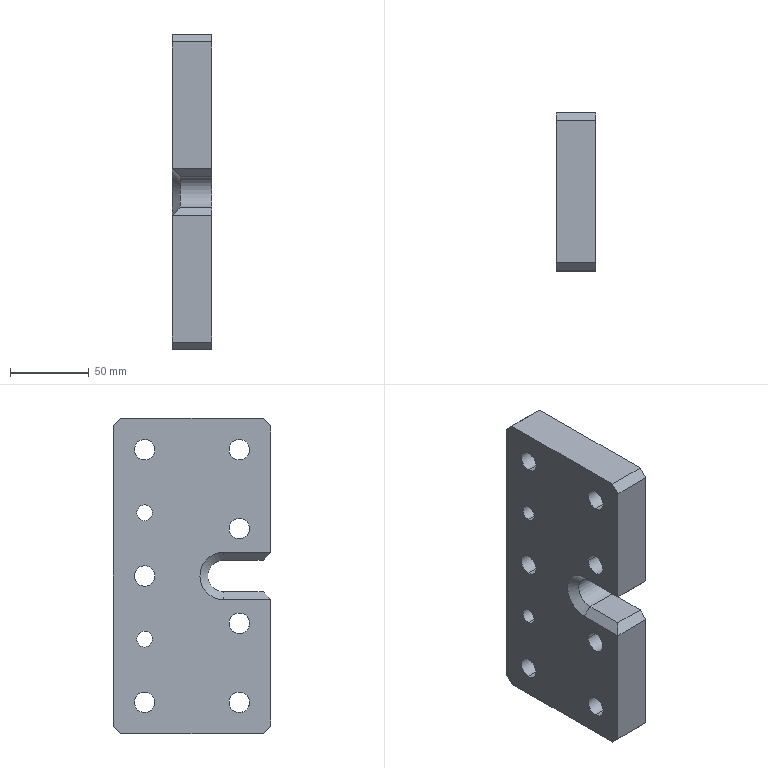Part | STEP file | Positioning_id646_x_t | 1 solid | 58 faces | box 25 x 100 x 200 mm | volume 431868 mm3 | cylinder 33 | plane 24 | cone 1 | commonest cylinder face diameters 20 x15 13 x14 10 x4